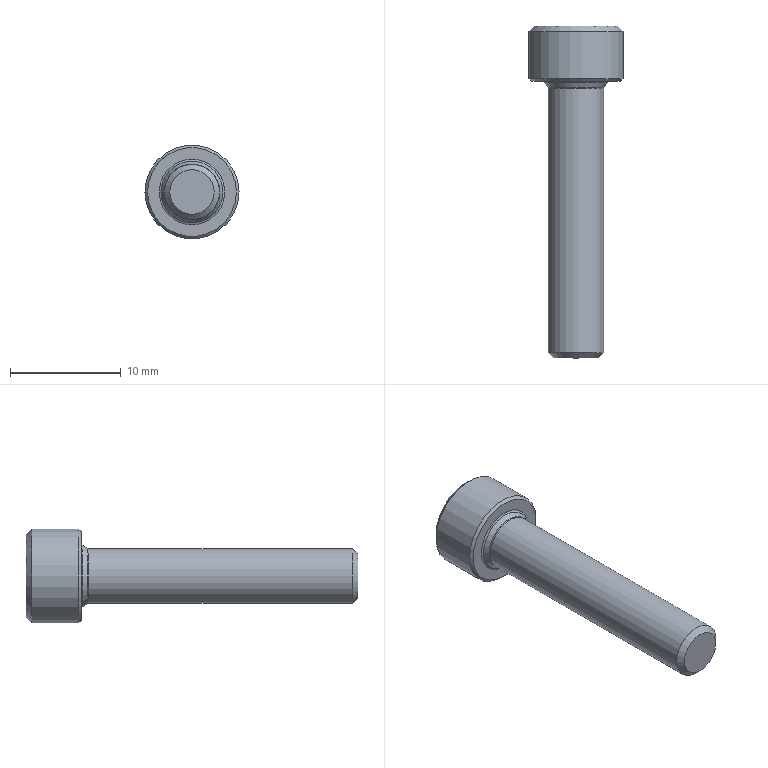Part | STEP file | 1 solid | 31 faces | box 8.5 x 30 x 8.5 mm | volume 723.48 mm3 | plane 15 | cone 11 | cylinder 3 | torus 2 | commonest cylinder face diameters 4 x1 5 x1 8.5 x1